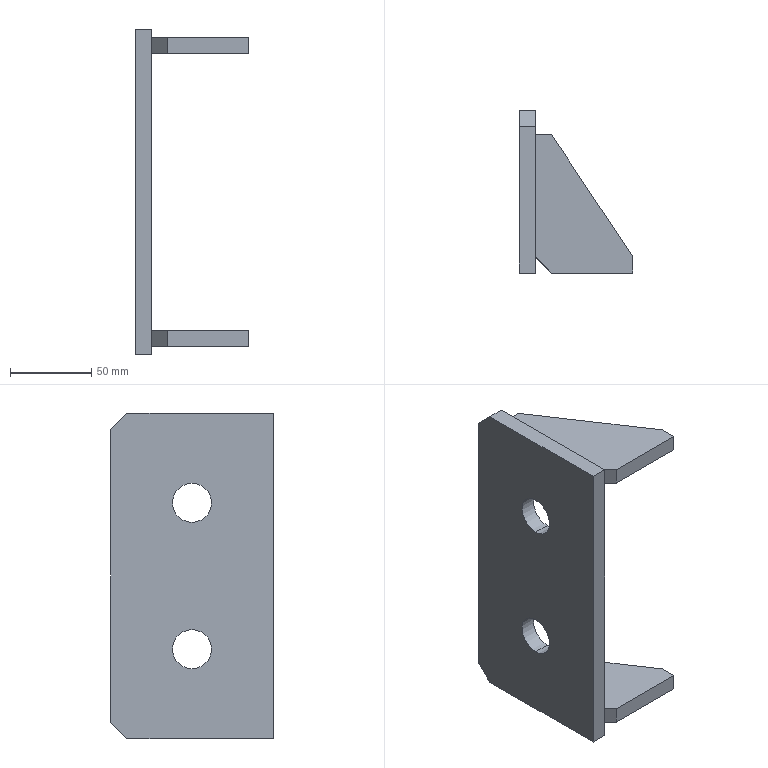Part | SolidWorks | 3 solids | 28 faces | box 70 x 100 x 200 mm | volume 253452 mm3 | plane 24 | cylinder 4 | commonest cylinder face diameters 24 x4
STEP:
#1=CARTESIAN_POINT('',(-10.,0.,33.));
#2=VERTEX_POINT('',#1);
#3=CARTESIAN_POINT('',(-10.,0.,57.));
#4=VERTEX_POINT('',#3);
#5=CARTESIAN_POINT('',(-10.,0.,45.));
#6=DIRECTION('',(-1.,0.,0.));
#7=DIRECTION('',(0.,0.,-1.));
#8=AXIS2_PLACEMENT_3D('',#5,#6,#7);
#9=CIRCLE('',#8,12.);
#10=EDGE_CURVE('',#2,#4,#9,.T.);
#11=ORIENTED_EDGE('',*,*,#10,.T.);
#12=CARTESIAN_POINT('',(0.,0.,57.));
#13=VERTEX_POINT('',#12);
#14=CARTESIAN_POINT('',(-10.001,0.,57.));
#15=DIRECTION('',(1.,0.,0.));
#16=VECTOR('',#15,1000.);
#17=LINE('',#14,#16);
#18=EDGE_CURVE('',#4,#13,#17,.T.);
#19=ORIENTED_EDGE('',*,*,#18,.T.);
#20=CARTESIAN_POINT('',(0.,0.,33.));
#21=VERTEX_POINT('',#20);
#22=CARTESIAN_POINT('',(0.,0.,45.));
#23=DIRECTION('',(1.,0.,0.));
#24=DIRECTION('',(0.,0.,-1.));
#25=AXIS2_PLACEMENT_3D('',#22,#23,#24);
#26=CIRCLE('',#25,12.);
#27=EDGE_CURVE('',#13,#21,#26,.T.);
#28=ORIENTED_EDGE('',*,*,#27,.T.);
#29=CARTESIAN_POINT('',(-10.001,0.,33.));
#30=DIRECTION('',(1.,0.,0.));
#31=VECTOR('',#30,1000.);
#32=LINE('',#29,#31);
#33=EDGE_CURVE('',#2,#21,#32,.T.);
#34=ORIENTED_EDGE('',*,*,#33,.F.);
#35=EDGE_LOOP('',(#11,#19,#28,#34));
#36=FACE_OUTER_BOUND('',#35,.T.);
#37=CARTESIAN_POINT('',(-10.001,0.,45.));
#38=DIRECTION('',(1.,0.,0.));
#39=DIRECTION('',(0.,0.,-1.));
#40=AXIS2_PLACEMENT_3D('',#37,#38,#39);
#41=CYLINDRICAL_SURFACE('',#40,12.);
#42=ADVANCED_FACE('',(#36),#41,.F.);
#43=CARTESIAN_POINT('',(-10.,0.,-57.));
#44=VERTEX_POINT('',#43);
#45=CARTESIAN_POINT('',(-10.,0.,-33.));
#46=VERTEX_POINT('',#45);
#47=CARTESIAN_POINT('',(-10.,0.,-45.));
#48=DIRECTION('',(-1.,0.,0.));
#49=DIRECTION('',(0.,0.,-1.));
#50=AXIS2_PLACEMENT_3D('',#47,#48,#49);
#51=CIRCLE('',#50,12.);
#52=EDGE_CURVE('',#44,#46,#51,.T.);
#53=ORIENTED_EDGE('',*,*,#52,.T.);
#54=CARTESIAN_POINT('',(0.,0.,-33.));
#55=VERTEX_POINT('',#54);
#56=CARTESIAN_POINT('',(-10.001,0.,-33.));
#57=DIRECTION('',(1.,0.,0.));
#58=VECTOR('',#57,1000.);
#59=LINE('',#56,#58);
#60=EDGE_CURVE('',#46,#55,#59,.T.);
#61=ORIENTED_EDGE('',*,*,#60,.T.);
#62=CARTESIAN_POINT('',(0.,0.,-57.));
#63=VERTEX_POINT('',#62);
#64=CARTESIAN_POINT('',(0.,0.,-45.));
#65=DIRECTION('',(1.,0.,0.));
#66=DIRECTION('',(0.,0.,1.));
#67=AXIS2_PLACEMENT_3D('',#64,#65,#66);
#68=CIRCLE('',#67,12.);
#69=EDGE_CURVE('',#55,#63,#68,.T.);
#70=ORIENTED_EDGE('',*,*,#69,.T.);
#71=CARTESIAN_POINT('',(-10.001,0.,-57.));
#72=DIRECTION('',(1.,0.,0.));
#73=VECTOR('',#72,1000.);
#74=LINE('',#71,#73);
#75=EDGE_CURVE('',#44,#63,#74,.T.);
#76=ORIENTED_EDGE('',*,*,#75,.F.);
#77=EDGE_LOOP('',(#53,#61,#70,#76));
#78=FACE_OUTER_BOUND('',#77,.T.);
#79=CARTESIAN_POINT('',(-10.001,0.,-45.));
#80=DIRECTION('',(1.,0.,0.));
#81=DIRECTION('',(0.,0.,-1.));
#82=AXIS2_PLACEMENT_3D('',#79,#80,#81);
#83=CYLINDRICAL_SURFACE('',#82,12.);
#84=ADVANCED_FACE('',(#78),#83,.F.);
#85=CARTESIAN_POINT('',(0.,40.,100.));
#86=VERTEX_POINT('',#85);
#87=CARTESIAN_POINT('',(0.,-50.,100.));
#88=VERTEX_POINT('',#87);
#89=CARTESIAN_POINT('',(0.,-50.,100.));
#90=DIRECTION('',(0.,-1.,0.));
#91=VECTOR('',#90,1000.);
#92=LINE('',#89,#91);
#93=EDGE_CURVE('',#86,#88,#92,.T.);
#94=ORIENTED_EDGE('',*,*,#93,.F.);
#95=CARTESIAN_POINT('',(-10.,40.,100.));
#96=VERTEX_POINT('',#95);
#97=CARTESIAN_POINT('',(-10.,40.,100.));
#98=DIRECTION('',(-1.,0.,0.));
#99=VECTOR('',#98,1000.);
#100=LINE('',#97,#99);
#101=EDGE_CURVE('',#86,#96,#100,.T.);
#102=ORIENTED_EDGE('',*,*,#101,.T.);
#103=CARTESIAN_POINT('',(-10.,-50.,100.));
#104=VERTEX_POINT('',#103);
#105=CARTESIAN_POINT('',(-10.,-50.,100.));
#106=DIRECTION('',(0.,-1.,0.));
#107=VECTOR('',#106,1000.);
#108=LINE('',#105,#107);
#109=EDGE_CURVE('',#96,#104,#108,.T.);
#110=ORIENTED_EDGE('',*,*,#109,.T.);
#111=CARTESIAN_POINT('',(-10.,-50.,100.));
#112=DIRECTION('',(1.,0.,0.));
#113=VECTOR('',#112,1000.);
#114=LINE('',#111,#113);
#115=EDGE_CURVE('',#104,#88,#114,.T.);
#116=ORIENTED_EDGE('',*,*,#115,.T.);
#117=EDGE_LOOP('',(#94,#102,#110,#116));
#118=FACE_OUTER_BOUND('',#117,.T.);
#119=CARTESIAN_POINT('',(-10.,-50.,100.));
#120=DIRECTION('',(0.,0.,1.));
#121=DIRECTION('',(1.,0.,0.));
#122=AXIS2_PLACEMENT_3D('',#119,#120,#121);
#123=PLANE('',#122);
#124=ADVANCED_FACE('',(#118),#123,.T.);
#125=CARTESIAN_POINT('',(0.,50.,-90.));
#126=VERTEX_POINT('',#125);
#127=CARTESIAN_POINT('',(0.,50.,90.));
#128=VERTEX_POINT('',#127);
#129=CARTESIAN_POINT('',(0.,50.,-100.));
#130=DIRECTION('',(0.,0.,1.));
#131=VECTOR('',#130,1000.);
#132=LINE('',#129,#131);
#133=EDGE_CURVE('',#126,#128,#132,.T.);
#134=ORIENTED_EDGE('',*,*,#133,.F.);
#135=CARTESIAN_POINT('',(-10.,50.,-90.));
#136=VERTEX_POINT('',#135);
#137=CARTESIAN_POINT('',(-10.,50.,-90.));
#138=DIRECTION('',(-1.,0.,0.));
#139=VECTOR('',#138,1000.);
#140=LINE('',#137,#139);
#141=EDGE_CURVE('',#126,#136,#140,.T.);
#142=ORIENTED_EDGE('',*,*,#141,.T.);
#143=CARTESIAN_POINT('',(-10.,50.,90.));
#144=VERTEX_POINT('',#143);
#145=CARTESIAN_POINT('',(-10.,50.,-100.));
#146=DIRECTION('',(0.,0.,1.));
#147=VECTOR('',#146,1000.);
#148=LINE('',#145,#147);
#149=EDGE_CURVE('',#136,#144,#148,.T.);
#150=ORIENTED_EDGE('',*,*,#149,.T.);
#151=CARTESIAN_POINT('',(-10.,50.,90.));
#152=DIRECTION('',(1.,0.,0.));
#153=VECTOR('',#152,1000.);
#154=LINE('',#151,#153);
#155=EDGE_CURVE('',#144,#128,#154,.T.);
#156=ORIENTED_EDGE('',*,*,#155,.T.);
#157=EDGE_LOOP('',(#134,#142,#150,#156));
#158=FACE_OUTER_BOUND('',#157,.T.);
#159=CARTESIAN_POINT('',(-10.,50.,-100.));
#160=DIRECTION('',(0.,1.,0.));
#161=DIRECTION('',(0.,0.,1.));
#162=AXIS2_PLACEMENT_3D('',#159,#160,#161);
#163=PLANE('',#162);
#164=ADVANCED_FACE('',(#158),#163,.T.);
#165=CARTESIAN_POINT('',(-10.,-50.,-100.));
#166=VERTEX_POINT('',#165);
#167=CARTESIAN_POINT('',(-10.,40.,-100.));
#168=VERTEX_POINT('',#167);
#169=CARTESIAN_POINT('',(-10.,-50.,-100.));
#170=DIRECTION('',(0.,1.,0.));
#171=VECTOR('',#170,1000.);
#172=LINE('',#169,#171);
#173=EDGE_CURVE('',#166,#168,#172,.T.);
#174=ORIENTED_EDGE('',*,*,#173,.T.);
#175=CARTESIAN_POINT('',(0.,40.,-100.));
#176=VERTEX_POINT('',#175);
#177=CARTESIAN_POINT('',(-10.,40.,-100.));
#178=DIRECTION('',(1.,0.,0.));
#179=VECTOR('',#178,1000.);
#180=LINE('',#177,#179);
#181=EDGE_CURVE('',#168,#176,#180,.T.);
#182=ORIENTED_EDGE('',*,*,#181,.T.);
#183=CARTESIAN_POINT('',(0.,-50.,-100.));
#184=VERTEX_POINT('',#183);
#185=CARTESIAN_POINT('',(0.,-50.,-100.));
#186=DIRECTION('',(0.,1.,0.));
#187=VECTOR('',#186,1000.);
#188=LINE('',#185,#187);
#189=EDGE_CURVE('',#184,#176,#188,.T.);
#190=ORIENTED_EDGE('',*,*,#189,.F.);
#191=CARTESIAN_POINT('',(-10.,-50.,-100.));
#192=DIRECTION('',(1.,0.,0.));
#193=VECTOR('',#192,1000.);
#194=LINE('',#191,#193);
#195=EDGE_CURVE('',#166,#184,#194,.T.);
#196=ORIENTED_EDGE('',*,*,#195,.F.);
#197=EDGE_LOOP('',(#174,#182,#190,#196));
#198=FACE_OUTER_BOUND('',#197,.T.);
#199=CARTESIAN_POINT('',(-10.,-50.,-100.));
#200=DIRECTION('',(0.,0.,-1.));
#201=DIRECTION('',(0.,1.,0.));
#202=AXIS2_PLACEMENT_3D('',#199,#200,#201);
#203=PLANE('',#202);
#204=ADVANCED_FACE('',(#198),#203,.T.);
#205=CARTESIAN_POINT('',(0.,-50.,-100.));
#206=DIRECTION('',(0.,0.,-1.));
#207=VECTOR('',#206,1000.);
#208=LINE('',#205,#207);
#209=EDGE_CURVE('',#88,#184,#208,.T.);
#210=ORIENTED_EDGE('',*,*,#209,.F.);
#211=ORIENTED_EDGE('',*,*,#115,.F.);
#212=CARTESIAN_POINT('',(-10.,-50.,-100.));
#213=DIRECTION('',(0.,0.,-1.));
#214=VECTOR('',#213,1000.);
#215=LINE('',#212,#214);
#216=EDGE_CURVE('',#104,#166,#215,.T.);
#217=ORIENTED_EDGE('',*,*,#216,.T.);
#218=ORIENTED_EDGE('',*,*,#195,.T.);
#219=EDGE_LOOP('',(#210,#211,#217,#218));
#220=FACE_OUTER_BOUND('',#219,.T.);
#221=CARTESIAN_POINT('',(-10.,-50.,-100.));
#222=DIRECTION('',(0.,-1.,0.));
#223=DIRECTION('',(0.,0.,-1.));
#224=AXIS2_PLACEMENT_3D('',#221,#222,#223);
#225=PLANE('',#224);
#226=ADVANCED_FACE('',(#220),#225,.T.);
#227=ORIENTED_EDGE('',*,*,#10,.F.);
#228=CARTESIAN_POINT('',(-10.,0.,45.));
#229=DIRECTION('',(-1.,0.,0.));
#230=DIRECTION('',(0.,0.,-1.));
#231=AXIS2_PLACEMENT_3D('',#228,#229,#230);
#232=CIRCLE('',#231,12.);
#233=EDGE_CURVE('',#4,#2,#232,.T.);
#234=ORIENTED_EDGE('',*,*,#233,.F.);
#235=EDGE_LOOP('',(#227,#234));
#236=FACE_BOUND('',#235,.T.);
#237=ORIENTED_EDGE('',*,*,#52,.F.);
#238=CARTESIAN_POINT('',(-10.,0.,-45.));
#239=DIRECTION('',(-1.,0.,0.));
#240=DIRECTION('',(0.,0.,-1.));
#241=AXIS2_PLACEMENT_3D('',#238,#239,#240);
#242=CIRCLE('',#241,12.);
#243=EDGE_CURVE('',#46,#44,#242,.T.);
#244=ORIENTED_EDGE('',*,*,#243,.F.);
#245=EDGE_LOOP('',(#237,#244));
#246=FACE_BOUND('',#245,.T.);
#247=ORIENTED_EDGE('',*,*,#149,.F.);
#248=CARTESIAN_POINT('',(-10.,40.,-100.));
#249=DIRECTION('',(0.,-0.7071,-0.7071));
#250=VECTOR('',#249,1000.);
#251=LINE('',#248,#250);
#252=EDGE_CURVE('',#136,#168,#251,.T.);
#253=ORIENTED_EDGE('',*,*,#252,.T.);
#254=ORIENTED_EDGE('',*,*,#173,.F.);
#255=ORIENTED_EDGE('',*,*,#216,.F.);
#256=ORIENTED_EDGE('',*,*,#109,.F.);
#257=CARTESIAN_POINT('',(-10.,50.,90.));
#258=DIRECTION('',(0.,0.7071,-0.7071));
#259=VECTOR('',#258,1000.);
#260=LINE('',#257,#259);
#261=EDGE_CURVE('',#96,#144,#260,.T.);
#262=ORIENTED_EDGE('',*,*,#261,.T.);
#263=EDGE_LOOP('',(#247,#253,#254,#255,#256,#262));
#264=FACE_OUTER_BOUND('',#263,.T.);
#265=CARTESIAN_POINT('',(-10.,0.,0.));
#266=DIRECTION('',(1.,0.,0.));
#267=DIRECTION('',(0.,0.,-1.));
#268=AXIS2_PLACEMENT_3D('',#265,#266,#267);
#269=PLANE('',#268);
#270=ADVANCED_FACE('',(#236,#246,#264),#269,.F.);
#271=CARTESIAN_POINT('',(0.,0.,45.));
#272=DIRECTION('',(1.,0.,0.));
#273=DIRECTION('',(0.,0.,-1.));
#274=AXIS2_PLACEMENT_3D('',#271,#272,#273);
#275=CIRCLE('',#274,12.);
#276=EDGE_CURVE('',#21,#13,#275,.T.);
#277=ORIENTED_EDGE('',*,*,#276,.F.);
#278=ORIENTED_EDGE('',*,*,#27,.F.);
#279=EDGE_LOOP('',(#277,#278));
#280=FACE_BOUND('',#279,.T.);
#281=CARTESIAN_POINT('',(0.,0.,-45.));
#282=DIRECTION('',(1.,0.,0.));
#283=DIRECTION('',(0.,0.,1.));
#284=AXIS2_PLACEMENT_3D('',#281,#282,#283);
#285=CIRCLE('',#284,12.);
#286=EDGE_CURVE('',#63,#55,#285,.T.);
#287=ORIENTED_EDGE('',*,*,#286,.F.);
#288=ORIENTED_EDGE('',*,*,#69,.F.);
#289=EDGE_LOOP('',(#287,#288));
#290=FACE_BOUND('',#289,.T.);
#291=ORIENTED_EDGE('',*,*,#189,.T.);
#292=CARTESIAN_POINT('',(0.,70.,-70.));
#293=DIRECTION('',(0.,0.7071,0.7071));
#294=VECTOR('',#293,1000.);
#295=LINE('',#292,#294);
#296=EDGE_CURVE('',#176,#126,#295,.T.);
#297=ORIENTED_EDGE('',*,*,#296,.T.);
#298=ORIENTED_EDGE('',*,*,#133,.T.);
#299=CARTESIAN_POINT('',(0.,70.,70.));
#300=DIRECTION('',(0.,-0.7071,0.7071));
#301=VECTOR('',#300,1000.);
#302=LINE('',#299,#301);
#303=EDGE_CURVE('',#128,#86,#302,.T.);
#304=ORIENTED_EDGE('',*,*,#303,.T.);
#305=ORIENTED_EDGE('',*,*,#93,.T.);
#306=ORIENTED_EDGE('',*,*,#209,.T.);
#307=EDGE_LOOP('',(#291,#297,#298,#304,#305,#306));
#308=FACE_OUTER_BOUND('',#307,.T.);
#309=CARTESIAN_POINT('',(0.,0.,0.));
#310=DIRECTION('',(1.,0.,0.));
#311=DIRECTION('',(0.,0.,-1.));
#312=AXIS2_PLACEMENT_3D('',#309,#310,#311);
#313=PLANE('',#312);
#314=ADVANCED_FACE('',(#280,#290,#308),#313,.T.);
#315=ORIENTED_EDGE('',*,*,#60,.F.);
#316=ORIENTED_EDGE('',*,*,#243,.T.);
#317=ORIENTED_EDGE('',*,*,#75,.T.);
#318=ORIENTED_EDGE('',*,*,#286,.T.);
#319=EDGE_LOOP('',(#315,#316,#317,#318));
#320=FACE_OUTER_BOUND('',#319,.T.);
#321=CARTESIAN_POINT('',(-10.001,0.,-45.));
#322=DIRECTION('',(1.,0.,0.));
#323=DIRECTION('',(0.,0.,-1.));
#324=AXIS2_PLACEMENT_3D('',#321,#322,#323);
#325=CYLINDRICAL_SURFACE('',#324,12.);
#326=ADVANCED_FACE('',(#320),#325,.F.);
#327=ORIENTED_EDGE('',*,*,#18,.F.);
#328=ORIENTED_EDGE('',*,*,#233,.T.);
#329=ORIENTED_EDGE('',*,*,#33,.T.);
#330=ORIENTED_EDGE('',*,*,#276,.T.);
#331=EDGE_LOOP('',(#327,#328,#329,#330));
#332=FACE_OUTER_BOUND('',#331,.T.);
#333=CARTESIAN_POINT('',(-10.001,0.,45.));
#334=DIRECTION('',(1.,0.,0.));
#335=DIRECTION('',(0.,0.,-1.));
#336=AXIS2_PLACEMENT_3D('',#333,#334,#335);
#337=CYLINDRICAL_SURFACE('',#336,12.);
#338=ADVANCED_FACE('',(#332),#337,.F.);
#339=ORIENTED_EDGE('',*,*,#252,.F.);
#340=ORIENTED_EDGE('',*,*,#141,.F.);
#341=ORIENTED_EDGE('',*,*,#296,.F.);
#342=ORIENTED_EDGE('',*,*,#181,.F.);
#343=EDGE_LOOP('',(#339,#340,#341,#342));
#344=FACE_OUTER_BOUND('',#343,.T.);
#345=CARTESIAN_POINT('',(-10.,40.,-100.));
#346=DIRECTION('',(0.,-0.7071,0.7071));
#347=DIRECTION('',(1.,0.,0.));
#348=AXIS2_PLACEMENT_3D('',#345,#346,#347);
#349=PLANE('',#348);
#350=ADVANCED_FACE('',(#344),#349,.F.);
#351=ORIENTED_EDGE('',*,*,#261,.F.);
#352=ORIENTED_EDGE('',*,*,#101,.F.);
#353=ORIENTED_EDGE('',*,*,#303,.F.);
#354=ORIENTED_EDGE('',*,*,#155,.F.);
#355=EDGE_LOOP('',(#351,#352,#353,#354));
#356=FACE_OUTER_BOUND('',#355,.T.);
#357=CARTESIAN_POINT('',(-10.,50.,90.));
#358=DIRECTION('',(0.,-0.7071,-0.7071));
#359=DIRECTION('',(1.,0.,0.));
#360=AXIS2_PLACEMENT_3D('',#357,#358,#359);
#361=PLANE('',#360);
#362=ADVANCED_FACE('',(#356),#361,.F.);
#363=CLOSED_SHELL('',(#42,#84,#124,#164,#204,#226,#270,#314,#326,#338,#350,#362));
#364=MANIFOLD_SOLID_BREP('',#363);
#365=CARTESIAN_POINT('',(0.,-40.,95.));
#366=VERTEX_POINT('',#365);
#367=CARTESIAN_POINT('',(10.,-50.,95.));
#368=VERTEX_POINT('',#367);
#369=CARTESIAN_POINT('',(0.,-40.,95.));
#370=DIRECTION('',(0.7071,-0.7071,0.));
#371=VECTOR('',#370,1000.);
#372=LINE('',#369,#371);
#373=EDGE_CURVE('',#366,#368,#372,.T.);
#374=ORIENTED_EDGE('',*,*,#373,.F.);
#375=CARTESIAN_POINT('',(0.,-40.,85.));
#376=VERTEX_POINT('',#375);
#377=CARTESIAN_POINT('',(0.,-40.,85.));
#378=DIRECTION('',(0.,0.,1.));
#379=VECTOR('',#378,1000.);
#380=LINE('',#377,#379);
#381=EDGE_CURVE('',#376,#366,#380,.T.);
#382=ORIENTED_EDGE('',*,*,#381,.F.);
#383=CARTESIAN_POINT('',(10.,-50.,85.));
#384=VERTEX_POINT('',#383);
#385=CARTESIAN_POINT('',(0.,-40.,85.));
#386=DIRECTION('',(0.7071,-0.7071,0.));
#387=VECTOR('',#386,1000.);
#388=LINE('',#385,#387);
#389=EDGE_CURVE('',#376,#384,#388,.T.);
#390=ORIENTED_EDGE('',*,*,#389,.T.);
#391=CARTESIAN_POINT('',(10.,-50.,85.));
#392=DIRECTION('',(0.,0.,1.));
#393=VECTOR('',#392,1000.);
#394=LINE('',#391,#393);
#395=EDGE_CURVE('',#384,#368,#394,.T.);
#396=ORIENTED_EDGE('',*,*,#395,.T.);
#397=EDGE_LOOP('',(#374,#382,#390,#396));
#398=FACE_OUTER_BOUND('',#397,.T.);
#399=CARTESIAN_POINT('',(0.,-40.,85.));
#400=DIRECTION('',(-0.7071,-0.7071,0.));
#401=DIRECTION('',(0.7071,-0.7071,0.));
#402=AXIS2_PLACEMENT_3D('',#399,#400,#401);
#403=PLANE('',#402);
#404=ADVANCED_FACE('',(#398),#403,.T.);
#405=CARTESIAN_POINT('',(0.,35.,95.));
#406=VERTEX_POINT('',#405);
#407=CARTESIAN_POINT('',(0.,35.,95.));
#408=DIRECTION('',(0.,-1.,0.));
#409=VECTOR('',#408,1000.);
#410=LINE('',#407,#409);
#411=EDGE_CURVE('',#406,#366,#410,.T.);
#412=ORIENTED_EDGE('',*,*,#411,.F.);
#413=CARTESIAN_POINT('',(0.,35.,85.));
#414=VERTEX_POINT('',#413);
#415=CARTESIAN_POINT('',(0.,35.,85.));
#416=DIRECTION('',(0.,0.,1.));
#417=VECTOR('',#416,1000.);
#418=LINE('',#415,#417);
#419=EDGE_CURVE('',#414,#406,#418,.T.);
#420=ORIENTED_EDGE('',*,*,#419,.F.);
#421=CARTESIAN_POINT('',(0.,35.,85.));
#422=DIRECTION('',(0.,-1.,0.));
#423=VECTOR('',#422,1000.);
#424=LINE('',#421,#423);
#425=EDGE_CURVE('',#414,#376,#424,.T.);
#426=ORIENTED_EDGE('',*,*,#425,.T.);
#427=ORIENTED_EDGE('',*,*,#381,.T.);
#428=EDGE_LOOP('',(#412,#420,#426,#427));
#429=FACE_OUTER_BOUND('',#428,.T.);
#430=CARTESIAN_POINT('',(0.,35.,85.));
#431=DIRECTION('',(-1.,0.,0.));
#432=DIRECTION('',(0.,0.,1.));
#433=AXIS2_PLACEMENT_3D('',#430,#431,#432);
#434=PLANE('',#433);
#435=ADVANCED_FACE('',(#429),#434,.T.);
#436=CARTESIAN_POINT('',(10.,35.,95.));
#437=VERTEX_POINT('',#436);
#438=CARTESIAN_POINT('',(10.,35.,95.));
#439=DIRECTION('',(-1.,0.,0.));
#440=VECTOR('',#439,1000.);
#441=LINE('',#438,#440);
#442=EDGE_CURVE('',#437,#406,#441,.T.);
#443=ORIENTED_EDGE('',*,*,#442,.F.);
#444=CARTESIAN_POINT('',(10.,35.,85.));
#445=VERTEX_POINT('',#444);
#446=CARTESIAN_POINT('',(10.,35.,85.));
#447=DIRECTION('',(0.,0.,1.));
#448=VECTOR('',#447,1000.);
#449=LINE('',#446,#448);
#450=EDGE_CURVE('',#445,#437,#449,.T.);
#451=ORIENTED_EDGE('',*,*,#450,.F.);
#452=CARTESIAN_POINT('',(10.,35.,85.));
#453=DIRECTION('',(-1.,0.,0.));
#454=VECTOR('',#453,1000.);
#455=LINE('',#452,#454);
#456=EDGE_CURVE('',#445,#414,#455,.T.);
#457=ORIENTED_EDGE('',*,*,#456,.T.);
#458=ORIENTED_EDGE('',*,*,#419,.T.);
#459=EDGE_LOOP('',(#443,#451,#457,#458));
#460=FACE_OUTER_BOUND('',#459,.T.);
#461=CARTESIAN_POINT('',(10.,35.,85.));
#462=DIRECTION('',(0.,1.,0.));
#463=DIRECTION('',(-1.,0.,0.));
#464=AXIS2_PLACEMENT_3D('',#461,#462,#463);
#465=PLANE('',#464);
#466=ADVANCED_FACE('',(#460),#465,.T.);
#467=CARTESIAN_POINT('',(60.,-40.,95.));
#468=VERTEX_POINT('',#467);
#469=CARTESIAN_POINT('',(60.,-40.,95.));
#470=DIRECTION('',(-0.5547,0.8321,0.));
#471=VECTOR('',#470,1000.);
#472=LINE('',#469,#471);
#473=EDGE_CURVE('',#468,#437,#472,.T.);
#474=ORIENTED_EDGE('',*,*,#473,.F.);
#475=CARTESIAN_POINT('',(60.,-40.,85.));
#476=VERTEX_POINT('',#475);
#477=CARTESIAN_POINT('',(60.,-40.,85.));
#478=DIRECTION('',(0.,0.,1.));
#479=VECTOR('',#478,1000.);
#480=LINE('',#477,#479);
#481=EDGE_CURVE('',#476,#468,#480,.T.);
#482=ORIENTED_EDGE('',*,*,#481,.F.);
#483=CARTESIAN_POINT('',(60.,-40.,85.));
#484=DIRECTION('',(-0.5547,0.8321,0.));
#485=VECTOR('',#484,1000.);
#486=LINE('',#483,#485);
#487=EDGE_CURVE('',#476,#445,#486,.T.);
#488=ORIENTED_EDGE('',*,*,#487,.T.);
#489=ORIENTED_EDGE('',*,*,#450,.T.);
#490=EDGE_LOOP('',(#474,#482,#488,#489));
#491=FACE_OUTER_BOUND('',#490,.T.);
#492=CARTESIAN_POINT('',(60.,-40.,85.));
#493=DIRECTION('',(0.8321,0.5547,0.));
#494=DIRECTION('',(-0.5547,0.8321,0.));
#495=AXIS2_PLACEMENT_3D('',#492,#493,#494);
#496=PLANE('',#495);
#497=ADVANCED_FACE('',(#491),#496,.T.);
#498=CARTESIAN_POINT('',(60.,-50.,95.));
#499=VERTEX_POINT('',#498);
#500=CARTESIAN_POINT('',(60.,-50.,95.));
#501=DIRECTION('',(0.,1.,0.));
#502=VECTOR('',#501,1000.);
#503=LINE('',#500,#502);
#504=EDGE_CURVE('',#499,#468,#503,.T.);
#505=ORIENTED_EDGE('',*,*,#504,.F.);
#506=CARTESIAN_POINT('',(60.,-50.,85.));
#507=VERTEX_POINT('',#506);
#508=CARTESIAN_POINT('',(60.,-50.,85.));
#509=DIRECTION('',(0.,0.,1.));
#510=VECTOR('',#509,1000.);
#511=LINE('',#508,#510);
#512=EDGE_CURVE('',#507,#499,#511,.T.);
#513=ORIENTED_EDGE('',*,*,#512,.F.);
#514=CARTESIAN_POINT('',(60.,-50.,85.));
#515=DIRECTION('',(0.,1.,0.));
#516=VECTOR('',#515,1000.);
#517=LINE('',#514,#516);
#518=EDGE_CURVE('',#507,#476,#517,.T.);
#519=ORIENTED_EDGE('',*,*,#518,.T.);
#520=ORIENTED_EDGE('',*,*,#481,.T.);
#521=EDGE_LOOP('',(#505,#513,#519,#520));
#522=FACE_OUTER_BOUND('',#521,.T.);
#523=CARTESIAN_POINT('',(60.,-50.,85.));
#524=DIRECTION('',(1.,0.,0.));
#525=DIRECTION('',(0.,0.,-1.));
#526=AXIS2_PLACEMENT_3D('',#523,#524,#525);
#527=PLANE('',#526);
#528=ADVANCED_FACE('',(#522),#527,.T.);
#529=CARTESIAN_POINT('',(10.,-50.,95.));
#530=DIRECTION('',(1.,0.,0.));
#531=VECTOR('',#530,1000.);
#532=LINE('',#529,#531);
#533=EDGE_CURVE('',#368,#499,#532,.T.);
#534=ORIENTED_EDGE('',*,*,#533,.F.);
#535=ORIENTED_EDGE('',*,*,#395,.F.);
#536=CARTESIAN_POINT('',(10.,-50.,85.));
#537=DIRECTION('',(1.,0.,0.));
#538=VECTOR('',#537,1000.);
#539=LINE('',#536,#538);
#540=EDGE_CURVE('',#384,#507,#539,.T.);
#541=ORIENTED_EDGE('',*,*,#540,.T.);
#542=ORIENTED_EDGE('',*,*,#512,.T.);
#543=EDGE_LOOP('',(#534,#535,#541,#542));
#544=FACE_OUTER_BOUND('',#543,.T.);
#545=CARTESIAN_POINT('',(10.,-50.,85.));
#546=DIRECTION('',(0.,-1.,0.));
#547=DIRECTION('',(0.,0.,-1.));
#548=AXIS2_PLACEMENT_3D('',#545,#546,#547);
#549=PLANE('',#548);
#550=ADVANCED_FACE('',(#544),#549,.T.);
#551=ORIENTED_EDGE('',*,*,#389,.F.);
#552=ORIENTED_EDGE('',*,*,#425,.F.);
#553=ORIENTED_EDGE('',*,*,#456,.F.);
#554=ORIENTED_EDGE('',*,*,#487,.F.);
#555=ORIENTED_EDGE('',*,*,#518,.F.);
#556=ORIENTED_EDGE('',*,*,#540,.F.);
#557=EDGE_LOOP('',(#551,#552,#553,#554,#555,#556));
#558=FACE_OUTER_BOUND('',#557,.T.);
#559=CARTESIAN_POINT('',(0.,0.,85.));
#560=DIRECTION('',(0.,0.,1.));
#561=DIRECTION('',(1.,0.,0.));
#562=AXIS2_PLACEMENT_3D('',#559,#560,#561);
#563=PLANE('',#562);
#564=ADVANCED_FACE('',(#558),#563,.F.);
#565=ORIENTED_EDGE('',*,*,#373,.T.);
#566=ORIENTED_EDGE('',*,*,#533,.T.);
#567=ORIENTED_EDGE('',*,*,#504,.T.);
#568=ORIENTED_EDGE('',*,*,#473,.T.);
#569=ORIENTED_EDGE('',*,*,#442,.T.);
#570=ORIENTED_EDGE('',*,*,#411,.T.);
#571=EDGE_LOOP('',(#565,#566,#567,#568,#569,#570));
#572=FACE_OUTER_BOUND('',#571,.T.);
#573=CARTESIAN_POINT('',(0.,0.,95.));
#574=DIRECTION('',(0.,0.,1.));
#575=DIRECTION('',(1.,0.,0.));
#576=AXIS2_PLACEMENT_3D('',#573,#574,#575);
#577=PLANE('',#576);
#578=ADVANCED_FACE('',(#572),#577,.T.);
#579=CLOSED_SHELL('',(#404,#435,#466,#497,#528,#550,#564,#578));
#580=MANIFOLD_SOLID_BREP('',#579);
#581=CARTESIAN_POINT('',(0.,-40.,-95.));
#582=VERTEX_POINT('',#581);
#583=CARTESIAN_POINT('',(10.,-50.,-95.));
#584=VERTEX_POINT('',#583);
#585=CARTESIAN_POINT('',(0.,-40.,-95.));
#586=DIRECTION('',(0.7071,-0.7071,0.));
#587=VECTOR('',#586,1000.);
#588=LINE('',#585,#587);
#589=EDGE_CURVE('',#582,#584,#588,.T.);
#590=ORIENTED_EDGE('',*,*,#589,.T.);
#591=CARTESIAN_POINT('',(10.,-50.,-85.));
#592=VERTEX_POINT('',#591);
#593=CARTESIAN_POINT('',(10.,-50.,-85.));
#594=DIRECTION('',(0.,0.,-1.));
#595=VECTOR('',#594,1000.);
#596=LINE('',#593,#595);
#597=EDGE_CURVE('',#592,#584,#596,.T.);
#598=ORIENTED_EDGE('',*,*,#597,.F.);
#599=CARTESIAN_POINT('',(0.,-40.,-85.));
#600=VERTEX_POINT('',#599);
#601=CARTESIAN_POINT('',(0.,-40.,-85.));
#602=DIRECTION('',(0.7071,-0.7071,0.));
#603=VECTOR('',#602,1000.);
#604=LINE('',#601,#603);
#605=EDGE_CURVE('',#600,#592,#604,.T.);
#606=ORIENTED_EDGE('',*,*,#605,.F.);
#607=CARTESIAN_POINT('',(0.,-40.,-85.));
#608=DIRECTION('',(0.,0.,-1.));
#609=VECTOR('',#608,1000.);
#610=LINE('',#607,#609);
#611=EDGE_CURVE('',#600,#582,#610,.T.);
#612=ORIENTED_EDGE('',*,*,#611,.T.);
#613=EDGE_LOOP('',(#590,#598,#606,#612));
#614=FACE_OUTER_BOUND('',#613,.T.);
#615=CARTESIAN_POINT('',(0.,-40.,-85.));
#616=DIRECTION('',(-0.7071,-0.7071,0.));
#617=DIRECTION('',(0.7071,-0.7071,0.));
#618=AXIS2_PLACEMENT_3D('',#615,#616,#617);
#619=PLANE('',#618);
#620=ADVANCED_FACE('',(#614),#619,.T.);
#621=CARTESIAN_POINT('',(0.,35.,-95.));
#622=VERTEX_POINT('',#621);
#623=CARTESIAN_POINT('',(0.,35.,-95.));
#624=DIRECTION('',(0.,-1.,0.));
#625=VECTOR('',#624,1000.);
#626=LINE('',#623,#625);
#627=EDGE_CURVE('',#622,#582,#626,.T.);
#628=ORIENTED_EDGE('',*,*,#627,.T.);
#629=ORIENTED_EDGE('',*,*,#611,.F.);
#630=CARTESIAN_POINT('',(0.,35.,-85.));
#631=VERTEX_POINT('',#630);
#632=CARTESIAN_POINT('',(0.,35.,-85.));
#633=DIRECTION('',(0.,-1.,0.));
#634=VECTOR('',#633,1000.);
#635=LINE('',#632,#634);
#636=EDGE_CURVE('',#631,#600,#635,.T.);
#637=ORIENTED_EDGE('',*,*,#636,.F.);
#638=CARTESIAN_POINT('',(0.,35.,-85.));
#639=DIRECTION('',(0.,0.,-1.));
#640=VECTOR('',#639,1000.);
#641=LINE('',#638,#640);
#642=EDGE_CURVE('',#631,#622,#641,.T.);
#643=ORIENTED_EDGE('',*,*,#642,.T.);
#644=EDGE_LOOP('',(#628,#629,#637,#643));
#645=FACE_OUTER_BOUND('',#644,.T.);
#646=CARTESIAN_POINT('',(0.,35.,-85.));
#647=DIRECTION('',(-1.,0.,0.));
#648=DIRECTION('',(0.,0.,-1.));
#649=AXIS2_PLACEMENT_3D('',#646,#647,#648);
#650=PLANE('',#649);
#651=ADVANCED_FACE('',(#645),#650,.T.);
#652=CARTESIAN_POINT('',(10.,35.,-95.));
#653=VERTEX_POINT('',#652);
#654=CARTESIAN_POINT('',(10.,35.,-95.));
#655=DIRECTION('',(-1.,0.,0.));
#656=VECTOR('',#655,1000.);
#657=LINE('',#654,#656);
#658=EDGE_CURVE('',#653,#622,#657,.T.);
#659=ORIENTED_EDGE('',*,*,#658,.T.);
#660=ORIENTED_EDGE('',*,*,#642,.F.);
#661=CARTESIAN_POINT('',(10.,35.,-85.));
#662=VERTEX_POINT('',#661);
#663=CARTESIAN_POINT('',(10.,35.,-85.));
#664=DIRECTION('',(-1.,0.,0.));
#665=VECTOR('',#664,1000.);
#666=LINE('',#663,#665);
#667=EDGE_CURVE('',#662,#631,#666,.T.);
#668=ORIENTED_EDGE('',*,*,#667,.F.);
#669=CARTESIAN_POINT('',(10.,35.,-85.));
#670=DIRECTION('',(0.,0.,-1.));
#671=VECTOR('',#670,1000.);
#672=LINE('',#669,#671);
#673=EDGE_CURVE('',#662,#653,#672,.T.);
#674=ORIENTED_EDGE('',*,*,#673,.T.);
#675=EDGE_LOOP('',(#659,#660,#668,#674));
#676=FACE_OUTER_BOUND('',#675,.T.);
#677=CARTESIAN_POINT('',(10.,35.,-85.));
#678=DIRECTION('',(0.,1.,0.));
#679=DIRECTION('',(-1.,0.,0.));
#680=AXIS2_PLACEMENT_3D('',#677,#678,#679);
#681=PLANE('',#680);
#682=ADVANCED_FACE('',(#676),#681,.T.);
#683=CARTESIAN_POINT('',(60.,-40.,-95.));
#684=VERTEX_POINT('',#683);
#685=CARTESIAN_POINT('',(60.,-40.,-95.));
#686=DIRECTION('',(-0.5547,0.8321,0.));
#687=VECTOR('',#686,1000.);
#688=LINE('',#685,#687);
#689=EDGE_CURVE('',#684,#653,#688,.T.);
#690=ORIENTED_EDGE('',*,*,#689,.T.);
#691=ORIENTED_EDGE('',*,*,#673,.F.);
#692=CARTESIAN_POINT('',(60.,-40.,-85.));
#693=VERTEX_POINT('',#692);
#694=CARTESIAN_POINT('',(60.,-40.,-85.));
#695=DIRECTION('',(-0.5547,0.8321,0.));
#696=VECTOR('',#695,1000.);
#697=LINE('',#694,#696);
#698=EDGE_CURVE('',#693,#662,#697,.T.);
#699=ORIENTED_EDGE('',*,*,#698,.F.);
#700=CARTESIAN_POINT('',(60.,-40.,-85.));
#701=DIRECTION('',(0.,0.,-1.));
#702=VECTOR('',#701,1000.);
#703=LINE('',#700,#702);
#704=EDGE_CURVE('',#693,#684,#703,.T.);
#705=ORIENTED_EDGE('',*,*,#704,.T.);
#706=EDGE_LOOP('',(#690,#691,#699,#705));
#707=FACE_OUTER_BOUND('',#706,.T.);
#708=CARTESIAN_POINT('',(60.,-40.,-85.));
#709=DIRECTION('',(0.8321,0.5547,0.));
#710=DIRECTION('',(-0.5547,0.8321,0.));
#711=AXIS2_PLACEMENT_3D('',#708,#709,#710);
#712=PLANE('',#711);
#713=ADVANCED_FACE('',(#707),#712,.T.);
#714=CARTESIAN_POINT('',(60.,-50.,-95.));
#715=VERTEX_POINT('',#714);
#716=CARTESIAN_POINT('',(60.,-50.,-95.));
#717=DIRECTION('',(0.,1.,0.));
#718=VECTOR('',#717,1000.);
#719=LINE('',#716,#718);
#720=EDGE_CURVE('',#715,#684,#719,.T.);
#721=ORIENTED_EDGE('',*,*,#720,.T.);
#722=ORIENTED_EDGE('',*,*,#704,.F.);
#723=CARTESIAN_POINT('',(60.,-50.,-85.));
#724=VERTEX_POINT('',#723);
#725=CARTESIAN_POINT('',(60.,-50.,-85.));
#726=DIRECTION('',(0.,1.,0.));
#727=VECTOR('',#726,1000.);
#728=LINE('',#725,#727);
#729=EDGE_CURVE('',#724,#693,#728,.T.);
#730=ORIENTED_EDGE('',*,*,#729,.F.);
#731=CARTESIAN_POINT('',(60.,-50.,-85.));
#732=DIRECTION('',(0.,0.,-1.));
#733=VECTOR('',#732,1000.);
#734=LINE('',#731,#733);
#735=EDGE_CURVE('',#724,#715,#734,.T.);
#736=ORIENTED_EDGE('',*,*,#735,.T.);
#737=EDGE_LOOP('',(#721,#722,#730,#736));
#738=FACE_OUTER_BOUND('',#737,.T.);
#739=CARTESIAN_POINT('',(60.,-50.,-85.));
#740=DIRECTION('',(1.,0.,0.));
#741=DIRECTION('',(0.,0.,1.));
#742=AXIS2_PLACEMENT_3D('',#739,#740,#741);
#743=PLANE('',#742);
#744=ADVANCED_FACE('',(#738),#743,.T.);
#745=CARTESIAN_POINT('',(10.,-50.,-95.));
#746=DIRECTION('',(1.,0.,0.));
#747=VECTOR('',#746,1000.);
#748=LINE('',#745,#747);
#749=EDGE_CURVE('',#584,#715,#748,.T.);
#750=ORIENTED_EDGE('',*,*,#749,.T.);
#751=ORIENTED_EDGE('',*,*,#735,.F.);
#752=CARTESIAN_POINT('',(10.,-50.,-85.));
#753=DIRECTION('',(1.,0.,0.));
#754=VECTOR('',#753,1000.);
#755=LINE('',#752,#754);
#756=EDGE_CURVE('',#592,#724,#755,.T.);
#757=ORIENTED_EDGE('',*,*,#756,.F.);
#758=ORIENTED_EDGE('',*,*,#597,.T.);
#759=EDGE_LOOP('',(#750,#751,#757,#758));
#760=FACE_OUTER_BOUND('',#759,.T.);
#761=CARTESIAN_POINT('',(10.,-50.,-85.));
#762=DIRECTION('',(0.,-1.,0.));
#763=DIRECTION('',(0.,0.,1.));
#764=AXIS2_PLACEMENT_3D('',#761,#762,#763);
#765=PLANE('',#764);
#766=ADVANCED_FACE('',(#760),#765,.T.);
#767=ORIENTED_EDGE('',*,*,#605,.T.);
#768=ORIENTED_EDGE('',*,*,#756,.T.);
#769=ORIENTED_EDGE('',*,*,#729,.T.);
#770=ORIENTED_EDGE('',*,*,#698,.T.);
#771=ORIENTED_EDGE('',*,*,#667,.T.);
#772=ORIENTED_EDGE('',*,*,#636,.T.);
#773=EDGE_LOOP('',(#767,#768,#769,#770,#771,#772));
#774=FACE_OUTER_BOUND('',#773,.T.);
#775=CARTESIAN_POINT('',(0.,0.,-85.));
#776=DIRECTION('',(0.,0.,-1.));
#777=DIRECTION('',(1.,0.,0.));
#778=AXIS2_PLACEMENT_3D('',#775,#776,#777);
#779=PLANE('',#778);
#780=ADVANCED_FACE('',(#774),#779,.F.);
#781=ORIENTED_EDGE('',*,*,#589,.F.);
#782=ORIENTED_EDGE('',*,*,#627,.F.);
#783=ORIENTED_EDGE('',*,*,#658,.F.);
#784=ORIENTED_EDGE('',*,*,#689,.F.);
#785=ORIENTED_EDGE('',*,*,#720,.F.);
#786=ORIENTED_EDGE('',*,*,#749,.F.);
#787=EDGE_LOOP('',(#781,#782,#783,#784,#785,#786));
#788=FACE_OUTER_BOUND('',#787,.T.);
#789=CARTESIAN_POINT('',(0.,0.,-95.));
#790=DIRECTION('',(0.,0.,-1.));
#791=DIRECTION('',(1.,0.,0.));
#792=AXIS2_PLACEMENT_3D('',#789,#790,#791);
#793=PLANE('',#792);
#794=ADVANCED_FACE('',(#788),#793,.T.);
#795=CLOSED_SHELL('',(#620,#651,#682,#713,#744,#766,#780,#794));
#796=MANIFOLD_SOLID_BREP('',#795);
#797=CARTESIAN_POINT('',(0.,0.,0.));
#798=DIRECTION('',(0.,0.,1.));
#799=DIRECTION('',(1.,0.,0.));
#800=AXIS2_PLACEMENT_3D('',#797,#798,#799);
#801=(LENGTH_UNIT()NAMED_UNIT(*)SI_UNIT(.MILLI.,.METRE.));
#802=UNCERTAINTY_MEASURE_WITH_UNIT(LENGTH_MEASURE(0.00001),#801,'','');
#803=(NAMED_UNIT(*)PLANE_ANGLE_UNIT()SI_UNIT($,.RADIAN.));
#804=(NAMED_UNIT(*)SI_UNIT($,.STERADIAN.)SOLID_ANGLE_UNIT());
#805=(GEOMETRIC_REPRESENTATION_CONTEXT(3)GLOBAL_UNCERTAINTY_ASSIGNED_CONTEXT((#802))GLOBAL_UNIT_ASSIGNED_CONTEXT((#801,#803,#804))REPRESENTATION_CONTEXT('',''));
#806=ADVANCED_BREP_SHAPE_REPRESENTATION('',(#364,#580,#796,#800),#805);